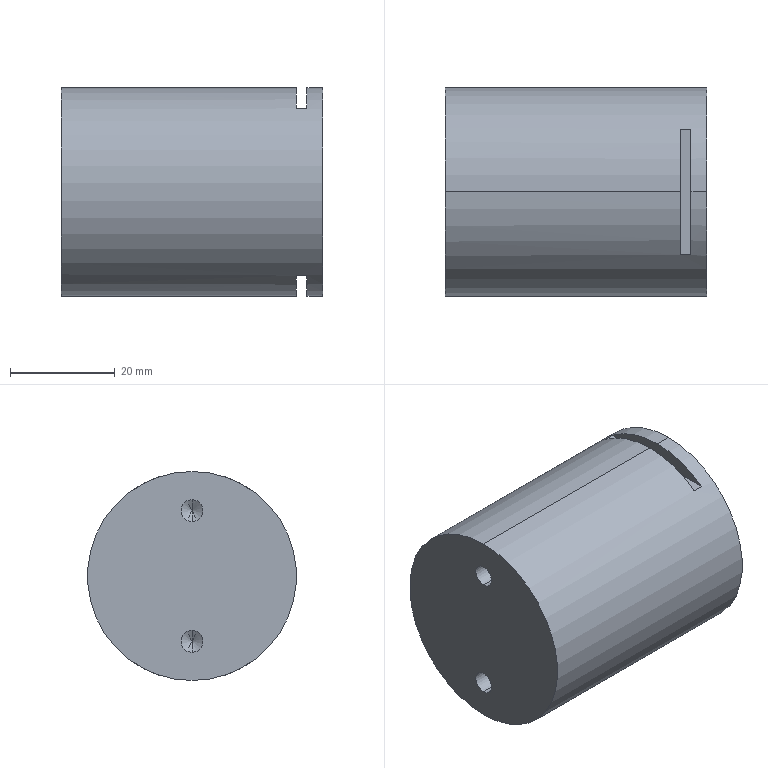Part | STEP file | 01-11 Coil feed support shaft | 1 solid | 18 faces | box 50 x 40 x 40 mm | volume 62215 mm3 | plane 8 | cylinder 6 | cone 4 | commonest cylinder face diameters 4.2 x4 40 x2
STEP:
#1=CARTESIAN_POINT('',(0.,0.,0.));
#2=DIRECTION('',(0.,0.,1.));
#3=DIRECTION('',(1.,0.,0.));
#4=AXIS2_PLACEMENT_3D('',#1,#2,#3);
#5=CARTESIAN_POINT('',(12.4,0.,-10.4));
#6=VERTEX_POINT('',#5);
#7=CARTESIAN_POINT('',(0.,0.,-10.4));
#8=VERTEX_POINT('',#7);
#9=CARTESIAN_POINT('',(12.4,0.,-10.4));
#10=DIRECTION('',(-1.,0.,0.));
#11=VECTOR('',#10,1.);
#12=LINE('',#9,#11);
#13=CARTESIAN_POINT('',(12.4,0.,-12.5));
#14=DIRECTION('',(-1.,0.,0.));
#15=DIRECTION('',(0.,0.,1.));
#16=AXIS2_PLACEMENT_3D('',#13,#14,#15);
#17=CYLINDRICAL_SURFACE('',#16,2.1);
#18=CARTESIAN_POINT('',(6.283,0.));
#19=DIRECTION('',(0.,1.));
#20=VECTOR('',#19,1.);
#21=LINE('',#18,#20);
#22=(GEOMETRIC_REPRESENTATION_CONTEXT(2)PARAMETRIC_REPRESENTATION_CONTEXT()REPRESENTATION_CONTEXT('',''));
#23=DEFINITIONAL_REPRESENTATION('',(#21),#22);
#24=PCURVE('',#17,#23);
#25=CARTESIAN_POINT('',(12.4,0.,-12.5));
#26=DIRECTION('',(-1.,0.,0.));
#27=DIRECTION('',(0.,0.,1.));
#28=AXIS2_PLACEMENT_3D('',#25,#26,#27);
#29=CYLINDRICAL_SURFACE('',#28,2.1);
#30=CARTESIAN_POINT('',(0.,0.));
#31=DIRECTION('',(0.,1.));
#32=VECTOR('',#31,1.);
#33=LINE('',#30,#32);
#34=(GEOMETRIC_REPRESENTATION_CONTEXT(2)PARAMETRIC_REPRESENTATION_CONTEXT()REPRESENTATION_CONTEXT('',''));
#35=DEFINITIONAL_REPRESENTATION('',(#33),#34);
#36=PCURVE('',#29,#35);
#37=SURFACE_CURVE('',#12,(#24,#36),.PCURVE_S1.);
#38=EDGE_CURVE('',#6,#8,#37,.T.);
#39=ORIENTED_EDGE('',*,*,#38,.T.);
#40=CARTESIAN_POINT('',(0.,0.,-14.6));
#41=VERTEX_POINT('',#40);
#42=CARTESIAN_POINT('',(0.,0.,-12.5));
#43=DIRECTION('',(-1.,0.,0.));
#44=DIRECTION('',(0.,0.,1.));
#45=AXIS2_PLACEMENT_3D('',#42,#43,#44);
#46=CIRCLE('',#45,2.1);
#47=CARTESIAN_POINT('',(0.,12.4));
#48=DIRECTION('',(1.,0.));
#49=VECTOR('',#48,1.);
#50=LINE('',#47,#49);
#51=(GEOMETRIC_REPRESENTATION_CONTEXT(2)PARAMETRIC_REPRESENTATION_CONTEXT()REPRESENTATION_CONTEXT('',''));
#52=DEFINITIONAL_REPRESENTATION('',(#50),#51);
#53=PCURVE('',#17,#52);
#54=CARTESIAN_POINT('',(0.,-20.24,20.24));
#55=DIRECTION('',(1.,0.,0.));
#56=DIRECTION('',(0.,0.,-1.));
#57=AXIS2_PLACEMENT_3D('',#54,#55,#56);
#58=PLANE('',#57);
#59=CARTESIAN_POINT('',(30.64,20.24));
#60=CARTESIAN_POINT('',(30.64,23.877));
#61=CARTESIAN_POINT('',(33.79,22.059));
#62=CARTESIAN_POINT('',(36.94,20.24));
#63=CARTESIAN_POINT('',(33.79,18.421));
#64=CARTESIAN_POINT('',(30.64,16.603));
#65=CARTESIAN_POINT('',(30.64,20.24));
#66=(BOUNDED_CURVE()B_SPLINE_CURVE(2,(#59,#60,#61,#62,#63,#64,#65),.UNSPECIFIED.,.T.,.F.)B_SPLINE_CURVE_WITH_KNOTS((1,2,2,2,2,1),(-2.094,0.,2.094,4.189,6.283,8.378),.UNSPECIFIED.)CURVE()GEOMETRIC_REPRESENTATION_ITEM()RATIONAL_B_SPLINE_CURVE((1.,0.5,1.,0.5,1.,0.5,1.))REPRESENTATION_ITEM(''));
#67=(GEOMETRIC_REPRESENTATION_CONTEXT(2)PARAMETRIC_REPRESENTATION_CONTEXT()REPRESENTATION_CONTEXT('',''));
#68=DEFINITIONAL_REPRESENTATION('',(#66),#67);
#69=PCURVE('',#58,#68);
#70=SURFACE_CURVE('',#46,(#53,#69),.PCURVE_S1.);
#71=EDGE_CURVE('',#41,#8,#70,.T.);
#72=ORIENTED_EDGE('',*,*,#71,.F.);
#73=CARTESIAN_POINT('',(12.4,0.,-14.6));
#74=VERTEX_POINT('',#73);
#75=CARTESIAN_POINT('',(12.4,0.,-14.6));
#76=DIRECTION('',(-1.,0.,0.));
#77=VECTOR('',#76,1.);
#78=LINE('',#75,#77);
#79=CARTESIAN_POINT('',(3.142,0.));
#80=DIRECTION('',(0.,1.));
#81=VECTOR('',#80,1.);
#82=LINE('',#79,#81);
#83=(GEOMETRIC_REPRESENTATION_CONTEXT(2)PARAMETRIC_REPRESENTATION_CONTEXT()REPRESENTATION_CONTEXT('',''));
#84=DEFINITIONAL_REPRESENTATION('',(#82),#83);
#85=PCURVE('',#17,#84);
#86=CARTESIAN_POINT('',(3.142,0.));
#87=DIRECTION('',(0.,1.));
#88=VECTOR('',#87,1.);
#89=LINE('',#86,#88);
#90=(GEOMETRIC_REPRESENTATION_CONTEXT(2)PARAMETRIC_REPRESENTATION_CONTEXT()REPRESENTATION_CONTEXT('',''));
#91=DEFINITIONAL_REPRESENTATION('',(#89),#90);
#92=PCURVE('',#29,#91);
#93=SURFACE_CURVE('',#78,(#85,#92),.PCURVE_S1.);
#94=EDGE_CURVE('',#74,#41,#93,.T.);
#95=ORIENTED_EDGE('',*,*,#94,.F.);
#96=CARTESIAN_POINT('',(12.4,0.,-12.5));
#97=DIRECTION('',(1.,0.,0.));
#98=DIRECTION('',(0.,0.,1.));
#99=AXIS2_PLACEMENT_3D('',#96,#97,#98);
#100=CIRCLE('',#99,2.1);
#101=CARTESIAN_POINT('',(6.283,0.));
#102=DIRECTION('',(-1.,0.));
#103=VECTOR('',#102,1.);
#104=LINE('',#101,#103);
#105=(GEOMETRIC_REPRESENTATION_CONTEXT(2)PARAMETRIC_REPRESENTATION_CONTEXT()REPRESENTATION_CONTEXT('',''));
#106=DEFINITIONAL_REPRESENTATION('',(#104),#105);
#107=PCURVE('',#17,#106);
#108=CARTESIAN_POINT('',(-986.338,0.,-12.5));
#109=DIRECTION('',(-1.,0.,0.));
#110=DIRECTION('',(0.,0.,1.));
#111=AXIS2_PLACEMENT_3D('',#108,#109,#110);
#112=CONICAL_SURFACE('',#111,1664.279,1.03);
#113=CARTESIAN_POINT('',(6.283,-998.738));
#114=DIRECTION('',(-1.,0.));
#115=VECTOR('',#114,1.);
#116=LINE('',#113,#115);
#117=(GEOMETRIC_REPRESENTATION_CONTEXT(2)PARAMETRIC_REPRESENTATION_CONTEXT()REPRESENTATION_CONTEXT('',''));
#118=DEFINITIONAL_REPRESENTATION('',(#116),#117);
#119=PCURVE('',#112,#118);
#120=SURFACE_CURVE('',#100,(#107,#119),.PCURVE_S1.);
#121=EDGE_CURVE('',#6,#74,#120,.T.);
#122=ORIENTED_EDGE('',*,*,#121,.F.);
#123=EDGE_LOOP('',(#39,#72,#95,#122));
#124=FACE_BOUND('',#123,.F.);
#125=ADVANCED_FACE('',(#124),#17,.F.);
#126=ORIENTED_EDGE('',*,*,#121,.T.);
#127=CARTESIAN_POINT('',(13.662,0.,-12.5));
#128=VERTEX_POINT('',#127);
#129=CARTESIAN_POINT('',(13.662,0.,-12.5));
#130=DIRECTION('',(-0.515,0.,-0.8572));
#131=VECTOR('',#130,1.);
#132=LINE('',#129,#131);
#133=CARTESIAN_POINT('',(3.142,-1000.));
#134=CARTESIAN_POINT('',(3.142,-999.981));
#135=CARTESIAN_POINT('',(3.142,-999.943));
#136=CARTESIAN_POINT('',(3.142,-999.885));
#137=CARTESIAN_POINT('',(3.142,-999.828));
#138=CARTESIAN_POINT('',(3.142,-999.771));
#139=CARTESIAN_POINT('',(3.142,-999.713));
#140=CARTESIAN_POINT('',(3.142,-999.656));
#141=CARTESIAN_POINT('',(3.142,-999.599));
#142=CARTESIAN_POINT('',(3.142,-999.541));
#143=CARTESIAN_POINT('',(3.142,-999.484));
#144=CARTESIAN_POINT('',(3.142,-999.426));
#145=CARTESIAN_POINT('',(3.142,-999.369));
#146=CARTESIAN_POINT('',(3.142,-999.312));
#147=CARTESIAN_POINT('',(3.142,-999.254));
#148=CARTESIAN_POINT('',(3.142,-999.197));
#149=CARTESIAN_POINT('',(3.142,-999.14));
#150=CARTESIAN_POINT('',(3.142,-999.082));
#151=CARTESIAN_POINT('',(3.142,-999.025));
#152=CARTESIAN_POINT('',(3.142,-998.968));
#153=CARTESIAN_POINT('',(3.142,-998.91));
#154=CARTESIAN_POINT('',(3.142,-998.853));
#155=CARTESIAN_POINT('',(3.142,-998.796));
#156=CARTESIAN_POINT('',(3.142,-998.757));
#157=CARTESIAN_POINT('',(3.142,-998.738));
#158=B_SPLINE_CURVE_WITH_KNOTS('',3,(#133,#134,#135,#136,#137,#138,#139,#140,#141,#142,#143,#144,#145,#146,#147,#148,#149,#150,#151,#152,#153,#154,#155,#156,#157),.UNSPECIFIED.,.F.,.F.,(4,1,1,1,1,1,1,1,1,1,1,1,1,1,1,1,1,1,1,1,1,1,4),(0.,0.1114,0.2227,0.3341,0.4454,0.5568,0.6682,0.7795,0.8909,1.002,1.114,1.225,1.336,1.448,1.559,1.67,1.782,1.893,2.004,2.116,2.227,2.339,2.45),.QUASI_UNIFORM_KNOTS.);
#159=(GEOMETRIC_REPRESENTATION_CONTEXT(2)PARAMETRIC_REPRESENTATION_CONTEXT()REPRESENTATION_CONTEXT('',''));
#160=DEFINITIONAL_REPRESENTATION('',(#158),#159);
#161=PCURVE('',#112,#160);
#162=CARTESIAN_POINT('',(-986.338,0.,-12.5));
#163=DIRECTION('',(-1.,0.,0.));
#164=DIRECTION('',(0.,0.,1.));
#165=AXIS2_PLACEMENT_3D('',#162,#163,#164);
#166=CONICAL_SURFACE('',#165,1664.279,1.03);
#167=CARTESIAN_POINT('',(3.142,-1000.));
#168=CARTESIAN_POINT('',(3.142,-999.981));
#169=CARTESIAN_POINT('',(3.142,-999.943));
#170=CARTESIAN_POINT('',(3.142,-999.885));
#171=CARTESIAN_POINT('',(3.142,-999.828));
#172=CARTESIAN_POINT('',(3.142,-999.771));
#173=CARTESIAN_POINT('',(3.142,-999.713));
#174=CARTESIAN_POINT('',(3.142,-999.656));
#175=CARTESIAN_POINT('',(3.142,-999.599));
#176=CARTESIAN_POINT('',(3.142,-999.541));
#177=CARTESIAN_POINT('',(3.142,-999.484));
#178=CARTESIAN_POINT('',(3.142,-999.426));
#179=CARTESIAN_POINT('',(3.142,-999.369));
#180=CARTESIAN_POINT('',(3.142,-999.312));
#181=CARTESIAN_POINT('',(3.142,-999.254));
#182=CARTESIAN_POINT('',(3.142,-999.197));
#183=CARTESIAN_POINT('',(3.142,-999.14));
#184=CARTESIAN_POINT('',(3.142,-999.082));
#185=CARTESIAN_POINT('',(3.142,-999.025));
#186=CARTESIAN_POINT('',(3.142,-998.968));
#187=CARTESIAN_POINT('',(3.142,-998.91));
#188=CARTESIAN_POINT('',(3.142,-998.853));
#189=CARTESIAN_POINT('',(3.142,-998.796));
#190=CARTESIAN_POINT('',(3.142,-998.757));
#191=CARTESIAN_POINT('',(3.142,-998.738));
#192=B_SPLINE_CURVE_WITH_KNOTS('',3,(#167,#168,#169,#170,#171,#172,#173,#174,#175,#176,#177,#178,#179,#180,#181,#182,#183,#184,#185,#186,#187,#188,#189,#190,#191),.UNSPECIFIED.,.F.,.F.,(4,1,1,1,1,1,1,1,1,1,1,1,1,1,1,1,1,1,1,1,1,1,4),(0.,0.1114,0.2227,0.3341,0.4454,0.5568,0.6682,0.7795,0.8909,1.002,1.114,1.225,1.336,1.448,1.559,1.67,1.782,1.893,2.004,2.116,2.227,2.339,2.45),.QUASI_UNIFORM_KNOTS.);
#193=(GEOMETRIC_REPRESENTATION_CONTEXT(2)PARAMETRIC_REPRESENTATION_CONTEXT()REPRESENTATION_CONTEXT('',''));
#194=DEFINITIONAL_REPRESENTATION('',(#192),#193);
#195=PCURVE('',#166,#194);
#196=SURFACE_CURVE('',#132,(#161,#195),.PCURVE_S1.);
#197=EDGE_CURVE('',#128,#74,#196,.T.);
#198=ORIENTED_EDGE('',*,*,#197,.F.);
#199=CARTESIAN_POINT('',(13.662,0.,-12.5));
#200=DIRECTION('',(-0.515,0.,0.8572));
#201=VECTOR('',#200,1.);
#202=LINE('',#199,#201);
#203=CARTESIAN_POINT('',(6.283,-1000.));
#204=DIRECTION('',(0.,1.));
#205=VECTOR('',#204,1.);
#206=LINE('',#203,#205);
#207=(GEOMETRIC_REPRESENTATION_CONTEXT(2)PARAMETRIC_REPRESENTATION_CONTEXT()REPRESENTATION_CONTEXT('',''));
#208=DEFINITIONAL_REPRESENTATION('',(#206),#207);
#209=PCURVE('',#112,#208);
#210=CARTESIAN_POINT('',(0.,-1000.));
#211=DIRECTION('',(0.,1.));
#212=VECTOR('',#211,1.);
#213=LINE('',#210,#212);
#214=(GEOMETRIC_REPRESENTATION_CONTEXT(2)PARAMETRIC_REPRESENTATION_CONTEXT()REPRESENTATION_CONTEXT('',''));
#215=DEFINITIONAL_REPRESENTATION('',(#213),#214);
#216=PCURVE('',#166,#215);
#217=SURFACE_CURVE('',#202,(#209,#216),.PCURVE_S1.);
#218=EDGE_CURVE('',#128,#6,#217,.T.);
#219=ORIENTED_EDGE('',*,*,#218,.T.);
#220=EDGE_LOOP('',(#126,#198,#219));
#221=FACE_BOUND('',#220,.F.);
#222=ADVANCED_FACE('',(#221),#112,.F.);
#223=CARTESIAN_POINT('',(12.4,0.,14.6));
#224=VERTEX_POINT('',#223);
#225=CARTESIAN_POINT('',(0.,0.,14.6));
#226=VERTEX_POINT('',#225);
#227=CARTESIAN_POINT('',(12.4,0.,14.6));
#228=DIRECTION('',(-1.,0.,0.));
#229=VECTOR('',#228,1.);
#230=LINE('',#227,#229);
#231=CARTESIAN_POINT('',(12.4,0.,12.5));
#232=DIRECTION('',(-1.,0.,0.));
#233=DIRECTION('',(0.,0.,1.));
#234=AXIS2_PLACEMENT_3D('',#231,#232,#233);
#235=CYLINDRICAL_SURFACE('',#234,2.1);
#236=CARTESIAN_POINT('',(6.283,0.));
#237=DIRECTION('',(0.,1.));
#238=VECTOR('',#237,1.);
#239=LINE('',#236,#238);
#240=(GEOMETRIC_REPRESENTATION_CONTEXT(2)PARAMETRIC_REPRESENTATION_CONTEXT()REPRESENTATION_CONTEXT('',''));
#241=DEFINITIONAL_REPRESENTATION('',(#239),#240);
#242=PCURVE('',#235,#241);
#243=CARTESIAN_POINT('',(12.4,0.,12.5));
#244=DIRECTION('',(-1.,0.,0.));
#245=DIRECTION('',(0.,0.,1.));
#246=AXIS2_PLACEMENT_3D('',#243,#244,#245);
#247=CYLINDRICAL_SURFACE('',#246,2.1);
#248=CARTESIAN_POINT('',(0.,0.));
#249=DIRECTION('',(0.,1.));
#250=VECTOR('',#249,1.);
#251=LINE('',#248,#250);
#252=(GEOMETRIC_REPRESENTATION_CONTEXT(2)PARAMETRIC_REPRESENTATION_CONTEXT()REPRESENTATION_CONTEXT('',''));
#253=DEFINITIONAL_REPRESENTATION('',(#251),#252);
#254=PCURVE('',#247,#253);
#255=SURFACE_CURVE('',#230,(#242,#254),.PCURVE_S1.);
#256=EDGE_CURVE('',#224,#226,#255,.T.);
#257=ORIENTED_EDGE('',*,*,#256,.T.);
#258=CARTESIAN_POINT('',(0.,0.,10.4));
#259=VERTEX_POINT('',#258);
#260=CARTESIAN_POINT('',(0.,0.,12.5));
#261=DIRECTION('',(-1.,0.,0.));
#262=DIRECTION('',(0.,0.,1.));
#263=AXIS2_PLACEMENT_3D('',#260,#261,#262);
#264=CIRCLE('',#263,2.1);
#265=CARTESIAN_POINT('',(0.,12.4));
#266=DIRECTION('',(1.,0.));
#267=VECTOR('',#266,1.);
#268=LINE('',#265,#267);
#269=(GEOMETRIC_REPRESENTATION_CONTEXT(2)PARAMETRIC_REPRESENTATION_CONTEXT()REPRESENTATION_CONTEXT('',''));
#270=DEFINITIONAL_REPRESENTATION('',(#268),#269);
#271=PCURVE('',#235,#270);
#272=CARTESIAN_POINT('',(5.64,20.24));
#273=CARTESIAN_POINT('',(5.64,23.877));
#274=CARTESIAN_POINT('',(8.79,22.059));
#275=CARTESIAN_POINT('',(11.94,20.24));
#276=CARTESIAN_POINT('',(8.79,18.421));
#277=CARTESIAN_POINT('',(5.64,16.603));
#278=CARTESIAN_POINT('',(5.64,20.24));
#279=(BOUNDED_CURVE()B_SPLINE_CURVE(2,(#272,#273,#274,#275,#276,#277,#278),.UNSPECIFIED.,.T.,.F.)B_SPLINE_CURVE_WITH_KNOTS((1,2,2,2,2,1),(-2.094,0.,2.094,4.189,6.283,8.378),.UNSPECIFIED.)CURVE()GEOMETRIC_REPRESENTATION_ITEM()RATIONAL_B_SPLINE_CURVE((1.,0.5,1.,0.5,1.,0.5,1.))REPRESENTATION_ITEM(''));
#280=(GEOMETRIC_REPRESENTATION_CONTEXT(2)PARAMETRIC_REPRESENTATION_CONTEXT()REPRESENTATION_CONTEXT('',''));
#281=DEFINITIONAL_REPRESENTATION('',(#279),#280);
#282=PCURVE('',#58,#281);
#283=SURFACE_CURVE('',#264,(#271,#282),.PCURVE_S1.);
#284=EDGE_CURVE('',#259,#226,#283,.T.);
#285=ORIENTED_EDGE('',*,*,#284,.F.);
#286=CARTESIAN_POINT('',(12.4,0.,10.4));
#287=VERTEX_POINT('',#286);
#288=CARTESIAN_POINT('',(12.4,0.,10.4));
#289=DIRECTION('',(-1.,0.,0.));
#290=VECTOR('',#289,1.);
#291=LINE('',#288,#290);
#292=CARTESIAN_POINT('',(3.142,0.));
#293=DIRECTION('',(0.,1.));
#294=VECTOR('',#293,1.);
#295=LINE('',#292,#294);
#296=(GEOMETRIC_REPRESENTATION_CONTEXT(2)PARAMETRIC_REPRESENTATION_CONTEXT()REPRESENTATION_CONTEXT('',''));
#297=DEFINITIONAL_REPRESENTATION('',(#295),#296);
#298=PCURVE('',#235,#297);
#299=CARTESIAN_POINT('',(3.142,0.));
#300=DIRECTION('',(0.,1.));
#301=VECTOR('',#300,1.);
#302=LINE('',#299,#301);
#303=(GEOMETRIC_REPRESENTATION_CONTEXT(2)PARAMETRIC_REPRESENTATION_CONTEXT()REPRESENTATION_CONTEXT('',''));
#304=DEFINITIONAL_REPRESENTATION('',(#302),#303);
#305=PCURVE('',#247,#304);
#306=SURFACE_CURVE('',#291,(#298,#305),.PCURVE_S1.);
#307=EDGE_CURVE('',#287,#259,#306,.T.);
#308=ORIENTED_EDGE('',*,*,#307,.F.);
#309=CARTESIAN_POINT('',(12.4,0.,12.5));
#310=DIRECTION('',(1.,0.,0.));
#311=DIRECTION('',(0.,0.,1.));
#312=AXIS2_PLACEMENT_3D('',#309,#310,#311);
#313=CIRCLE('',#312,2.1);
#314=CARTESIAN_POINT('',(6.283,0.));
#315=DIRECTION('',(-1.,0.));
#316=VECTOR('',#315,1.);
#317=LINE('',#314,#316);
#318=(GEOMETRIC_REPRESENTATION_CONTEXT(2)PARAMETRIC_REPRESENTATION_CONTEXT()REPRESENTATION_CONTEXT('',''));
#319=DEFINITIONAL_REPRESENTATION('',(#317),#318);
#320=PCURVE('',#235,#319);
#321=CARTESIAN_POINT('',(-986.338,0.,12.5));
#322=DIRECTION('',(-1.,0.,0.));
#323=DIRECTION('',(0.,0.,1.));
#324=AXIS2_PLACEMENT_3D('',#321,#322,#323);
#325=CONICAL_SURFACE('',#324,1664.279,1.03);
#326=CARTESIAN_POINT('',(6.283,-998.738));
#327=DIRECTION('',(-1.,0.));
#328=VECTOR('',#327,1.);
#329=LINE('',#326,#328);
#330=(GEOMETRIC_REPRESENTATION_CONTEXT(2)PARAMETRIC_REPRESENTATION_CONTEXT()REPRESENTATION_CONTEXT('',''));
#331=DEFINITIONAL_REPRESENTATION('',(#329),#330);
#332=PCURVE('',#325,#331);
#333=SURFACE_CURVE('',#313,(#320,#332),.PCURVE_S1.);
#334=EDGE_CURVE('',#224,#287,#333,.T.);
#335=ORIENTED_EDGE('',*,*,#334,.F.);
#336=EDGE_LOOP('',(#257,#285,#308,#335));
#337=FACE_BOUND('',#336,.F.);
#338=ADVANCED_FACE('',(#337),#235,.F.);
#339=CARTESIAN_POINT('',(50.,0.,-20.));
#340=VERTEX_POINT('',#339);
#341=CARTESIAN_POINT('',(50.,0.,20.));
#342=VERTEX_POINT('',#341);
#343=CARTESIAN_POINT('',(50.,0.,0.));
#344=DIRECTION('',(1.,0.,0.));
#345=DIRECTION('',(0.,0.,1.));
#346=AXIS2_PLACEMENT_3D('',#343,#344,#345);
#347=CIRCLE('',#346,20.);
#348=CARTESIAN_POINT('',(50.,0.,0.));
#349=DIRECTION('',(-1.,0.,0.));
#350=DIRECTION('',(0.,0.,1.));
#351=AXIS2_PLACEMENT_3D('',#348,#349,#350);
#352=CYLINDRICAL_SURFACE('',#351,20.);
#353=CARTESIAN_POINT('',(6.283,0.));
#354=DIRECTION('',(-1.,0.));
#355=VECTOR('',#354,1.);
#356=LINE('',#353,#355);
#357=(GEOMETRIC_REPRESENTATION_CONTEXT(2)PARAMETRIC_REPRESENTATION_CONTEXT()REPRESENTATION_CONTEXT('',''));
#358=DEFINITIONAL_REPRESENTATION('',(#356),#357);
#359=PCURVE('',#352,#358);
#360=CARTESIAN_POINT('',(50.,-20.24,20.24));
#361=DIRECTION('',(1.,0.,0.));
#362=DIRECTION('',(0.,0.,-1.));
#363=AXIS2_PLACEMENT_3D('',#360,#361,#362);
#364=PLANE('',#363);
#365=CARTESIAN_POINT('',(20.24,20.24));
#366=DIRECTION('',(-1.,0.));
#367=AXIS2_PLACEMENT_2D('',#365,#366);
#368=CIRCLE('',#367,20.);
#369=(GEOMETRIC_REPRESENTATION_CONTEXT(2)PARAMETRIC_REPRESENTATION_CONTEXT()REPRESENTATION_CONTEXT('',''));
#370=DEFINITIONAL_REPRESENTATION('',(#368),#369);
#371=PCURVE('',#364,#370);
#372=SURFACE_CURVE('',#347,(#359,#371),.PCURVE_S1.);
#373=EDGE_CURVE('',#340,#342,#372,.T.);
#374=ORIENTED_EDGE('',*,*,#373,.F.);
#375=CARTESIAN_POINT('',(47.,0.,-20.));
#376=VERTEX_POINT('',#375);
#377=CARTESIAN_POINT('',(50.,0.,-20.));
#378=DIRECTION('',(-1.,0.,0.));
#379=VECTOR('',#378,1.);
#380=LINE('',#377,#379);
#381=CARTESIAN_POINT('',(3.142,0.));
#382=DIRECTION('',(0.,1.));
#383=VECTOR('',#382,1.);
#384=LINE('',#381,#383);
#385=(GEOMETRIC_REPRESENTATION_CONTEXT(2)PARAMETRIC_REPRESENTATION_CONTEXT()REPRESENTATION_CONTEXT('',''));
#386=DEFINITIONAL_REPRESENTATION('',(#384),#385);
#387=PCURVE('',#352,#386);
#388=CARTESIAN_POINT('',(50.,0.,0.));
#389=DIRECTION('',(-1.,0.,0.));
#390=DIRECTION('',(0.,0.,1.));
#391=AXIS2_PLACEMENT_3D('',#388,#389,#390);
#392=CYLINDRICAL_SURFACE('',#391,20.);
#393=CARTESIAN_POINT('',(3.142,0.));
#394=DIRECTION('',(0.,1.));
#395=VECTOR('',#394,1.);
#396=LINE('',#393,#395);
#397=(GEOMETRIC_REPRESENTATION_CONTEXT(2)PARAMETRIC_REPRESENTATION_CONTEXT()REPRESENTATION_CONTEXT('',''));
#398=DEFINITIONAL_REPRESENTATION('',(#396),#397);
#399=PCURVE('',#392,#398);
#400=SURFACE_CURVE('',#380,(#387,#399),.PCURVE_S1.);
#401=EDGE_CURVE('',#340,#376,#400,.T.);
#402=ORIENTED_EDGE('',*,*,#401,.T.);
#403=CARTESIAN_POINT('',(47.,12.,-16.));
#404=VERTEX_POINT('',#403);
#405=CARTESIAN_POINT('',(47.,0.,0.));
#406=DIRECTION('',(-1.,0.,0.));
#407=DIRECTION('',(0.,0.,1.));
#408=AXIS2_PLACEMENT_3D('',#405,#406,#407);
#409=CIRCLE('',#408,20.);
#410=CARTESIAN_POINT('',(0.,3.));
#411=DIRECTION('',(1.,0.));
#412=VECTOR('',#411,1.);
#413=LINE('',#410,#412);
#414=(GEOMETRIC_REPRESENTATION_CONTEXT(2)PARAMETRIC_REPRESENTATION_CONTEXT()REPRESENTATION_CONTEXT('',''));
#415=DEFINITIONAL_REPRESENTATION('',(#413),#414);
#416=PCURVE('',#352,#415);
#417=CARTESIAN_POINT('',(47.,-12.144,-16.));
#418=DIRECTION('',(1.,0.,0.));
#419=DIRECTION('',(0.,0.,-1.));
#420=AXIS2_PLACEMENT_3D('',#417,#418,#419);
#421=PLANE('',#420);
#422=CARTESIAN_POINT('',(-36.,12.144));
#423=CARTESIAN_POINT('',(-36.,46.785));
#424=CARTESIAN_POINT('',(-6.,29.465));
#425=CARTESIAN_POINT('',(24.,12.144));
#426=CARTESIAN_POINT('',(-6.,-5.177));
#427=CARTESIAN_POINT('',(-36.,-22.497));
#428=CARTESIAN_POINT('',(-36.,12.144));
#429=(BOUNDED_CURVE()B_SPLINE_CURVE(2,(#422,#423,#424,#425,#426,#427,#428),.UNSPECIFIED.,.T.,.F.)B_SPLINE_CURVE_WITH_KNOTS((1,2,2,2,2,1),(-2.094,0.,2.094,4.189,6.283,8.378),.UNSPECIFIED.)CURVE()GEOMETRIC_REPRESENTATION_ITEM()RATIONAL_B_SPLINE_CURVE((1.,0.5,1.,0.5,1.,0.5,1.))REPRESENTATION_ITEM(''));
#430=(GEOMETRIC_REPRESENTATION_CONTEXT(2)PARAMETRIC_REPRESENTATION_CONTEXT()REPRESENTATION_CONTEXT('',''));
#431=DEFINITIONAL_REPRESENTATION('',(#429),#430);
#432=PCURVE('',#421,#431);
#433=SURFACE_CURVE('',#409,(#416,#432),.PCURVE_S1.);
#434=EDGE_CURVE('',#404,#376,#433,.T.);
#435=ORIENTED_EDGE('',*,*,#434,.F.);
#436=CARTESIAN_POINT('',(45.,12.,-16.));
#437=VERTEX_POINT('',#436);
#438=CARTESIAN_POINT('',(25.,12.,-16.));
#439=DIRECTION('',(1.,0.,0.));
#440=VECTOR('',#439,1.);
#441=LINE('',#438,#440);
#442=CARTESIAN_POINT('',(2.498,25.));
#443=DIRECTION('',(0.,-1.));
#444=VECTOR('',#443,1.);
#445=LINE('',#442,#444);
#446=(GEOMETRIC_REPRESENTATION_CONTEXT(2)PARAMETRIC_REPRESENTATION_CONTEXT()REPRESENTATION_CONTEXT('',''));
#447=DEFINITIONAL_REPRESENTATION('',(#445),#446);
#448=PCURVE('',#352,#447);
#449=CARTESIAN_POINT('',(45.,-12.,-16.));
#450=DIRECTION('',(0.,0.,1.));
#451=DIRECTION('',(1.,0.,0.));
#452=AXIS2_PLACEMENT_3D('',#449,#450,#451);
#453=PLANE('',#452);
#454=CARTESIAN_POINT('',(-20.,24.));
#455=DIRECTION('',(1.,0.));
#456=VECTOR('',#455,1.);
#457=LINE('',#454,#456);
#458=(GEOMETRIC_REPRESENTATION_CONTEXT(2)PARAMETRIC_REPRESENTATION_CONTEXT()REPRESENTATION_CONTEXT('',''));
#459=DEFINITIONAL_REPRESENTATION('',(#457),#458);
#460=PCURVE('',#453,#459);
#461=SURFACE_CURVE('',#441,(#448,#460),.PCURVE_S1.);
#462=EDGE_CURVE('',#437,#404,#461,.T.);
#463=ORIENTED_EDGE('',*,*,#462,.F.);
#464=CARTESIAN_POINT('',(45.,0.,-20.));
#465=VERTEX_POINT('',#464);
#466=CARTESIAN_POINT('',(45.,0.,0.));
#467=DIRECTION('',(1.,0.,0.));
#468=DIRECTION('',(0.,0.,1.));
#469=AXIS2_PLACEMENT_3D('',#466,#467,#468);
#470=CIRCLE('',#469,20.);
#471=CARTESIAN_POINT('',(6.283,5.));
#472=DIRECTION('',(-1.,0.));
#473=VECTOR('',#472,1.);
#474=LINE('',#471,#473);
#475=(GEOMETRIC_REPRESENTATION_CONTEXT(2)PARAMETRIC_REPRESENTATION_CONTEXT()REPRESENTATION_CONTEXT('',''));
#476=DEFINITIONAL_REPRESENTATION('',(#474),#475);
#477=PCURVE('',#352,#476);
#478=CARTESIAN_POINT('',(45.,-12.144,-20.024));
#479=DIRECTION('',(-1.,0.,0.));
#480=DIRECTION('',(0.,0.,1.));
#481=AXIS2_PLACEMENT_3D('',#478,#479,#480);
#482=PLANE('',#481);
#483=CARTESIAN_POINT('',(40.024,12.144));
#484=CARTESIAN_POINT('',(40.024,-22.497));
#485=CARTESIAN_POINT('',(10.024,-5.177));
#486=CARTESIAN_POINT('',(-19.976,12.144));
#487=CARTESIAN_POINT('',(10.024,29.465));
#488=CARTESIAN_POINT('',(40.024,46.785));
#489=CARTESIAN_POINT('',(40.024,12.144));
#490=(BOUNDED_CURVE()B_SPLINE_CURVE(2,(#483,#484,#485,#486,#487,#488,#489),.UNSPECIFIED.,.T.,.F.)B_SPLINE_CURVE_WITH_KNOTS((1,2,2,2,2,1),(-2.094,0.,2.094,4.189,6.283,8.378),.UNSPECIFIED.)CURVE()GEOMETRIC_REPRESENTATION_ITEM()RATIONAL_B_SPLINE_CURVE((1.,0.5,1.,0.5,1.,0.5,1.))REPRESENTATION_ITEM(''));
#491=(GEOMETRIC_REPRESENTATION_CONTEXT(2)PARAMETRIC_REPRESENTATION_CONTEXT()REPRESENTATION_CONTEXT('',''));
#492=DEFINITIONAL_REPRESENTATION('',(#490),#491);
#493=PCURVE('',#482,#492);
#494=SURFACE_CURVE('',#470,(#477,#493),.PCURVE_S1.);
#495=EDGE_CURVE('',#465,#437,#494,.T.);
#496=ORIENTED_EDGE('',*,*,#495,.F.);
#497=CARTESIAN_POINT('',(0.,0.,-20.));
#498=VERTEX_POINT('',#497);
#499=CARTESIAN_POINT('',(50.,0.,-20.));
#500=DIRECTION('',(-1.,0.,0.));
#501=VECTOR('',#500,1.);
#502=LINE('',#499,#501);
#503=CARTESIAN_POINT('',(3.142,0.));
#504=DIRECTION('',(0.,1.));
#505=VECTOR('',#504,1.);
#506=LINE('',#503,#505);
#507=(GEOMETRIC_REPRESENTATION_CONTEXT(2)PARAMETRIC_REPRESENTATION_CONTEXT()REPRESENTATION_CONTEXT('',''));
#508=DEFINITIONAL_REPRESENTATION('',(#506),#507);
#509=PCURVE('',#352,#508);
#510=CARTESIAN_POINT('',(3.142,0.));
#511=DIRECTION('',(0.,1.));
#512=VECTOR('',#511,1.);
#513=LINE('',#510,#512);
#514=(GEOMETRIC_REPRESENTATION_CONTEXT(2)PARAMETRIC_REPRESENTATION_CONTEXT()REPRESENTATION_CONTEXT('',''));
#515=DEFINITIONAL_REPRESENTATION('',(#513),#514);
#516=PCURVE('',#392,#515);
#517=SURFACE_CURVE('',#502,(#509,#516),.PCURVE_S1.);
#518=EDGE_CURVE('',#465,#498,#517,.T.);
#519=ORIENTED_EDGE('',*,*,#518,.T.);
#520=CARTESIAN_POINT('',(0.,0.,20.));
#521=VERTEX_POINT('',#520);
#522=CARTESIAN_POINT('',(0.,0.,0.));
#523=DIRECTION('',(1.,0.,0.));
#524=DIRECTION('',(0.,0.,1.));
#525=AXIS2_PLACEMENT_3D('',#522,#523,#524);
#526=CIRCLE('',#525,20.);
#527=CARTESIAN_POINT('',(6.283,50.));
#528=DIRECTION('',(-1.,0.));
#529=VECTOR('',#528,1.);
#530=LINE('',#527,#529);
#531=(GEOMETRIC_REPRESENTATION_CONTEXT(2)PARAMETRIC_REPRESENTATION_CONTEXT()REPRESENTATION_CONTEXT('',''));
#532=DEFINITIONAL_REPRESENTATION('',(#530),#531);
#533=PCURVE('',#352,#532);
#534=CARTESIAN_POINT('',(20.24,20.24));
#535=DIRECTION('',(-1.,0.));
#536=AXIS2_PLACEMENT_2D('',#534,#535);
#537=CIRCLE('',#536,20.);
#538=(GEOMETRIC_REPRESENTATION_CONTEXT(2)PARAMETRIC_REPRESENTATION_CONTEXT()REPRESENTATION_CONTEXT('',''));
#539=DEFINITIONAL_REPRESENTATION('',(#537),#538);
#540=PCURVE('',#58,#539);
#541=SURFACE_CURVE('',#526,(#533,#540),.PCURVE_S1.);
#542=EDGE_CURVE('',#498,#521,#541,.T.);
#543=ORIENTED_EDGE('',*,*,#542,.T.);
#544=CARTESIAN_POINT('',(45.,0.,20.));
#545=VERTEX_POINT('',#544);
#546=CARTESIAN_POINT('',(50.,0.,20.));
#547=DIRECTION('',(-1.,0.,0.));
#548=VECTOR('',#547,1.);
#549=LINE('',#546,#548);
#550=CARTESIAN_POINT('',(0.,0.));
#551=DIRECTION('',(0.,1.));
#552=VECTOR('',#551,1.);
#553=LINE('',#550,#552);
#554=(GEOMETRIC_REPRESENTATION_CONTEXT(2)PARAMETRIC_REPRESENTATION_CONTEXT()REPRESENTATION_CONTEXT('',''));
#555=DEFINITIONAL_REPRESENTATION('',(#553),#554);
#556=PCURVE('',#352,#555);
#557=CARTESIAN_POINT('',(6.283,0.));
#558=DIRECTION('',(0.,1.));
#559=VECTOR('',#558,1.);
#560=LINE('',#557,#559);
#561=(GEOMETRIC_REPRESENTATION_CONTEXT(2)PARAMETRIC_REPRESENTATION_CONTEXT()REPRESENTATION_CONTEXT('',''));
#562=DEFINITIONAL_REPRESENTATION('',(#560),#561);
#563=PCURVE('',#392,#562);
#564=SURFACE_CURVE('',#549,(#556,#563),.PCURVE_S1.);
#565=EDGE_CURVE('',#545,#521,#564,.T.);
#566=ORIENTED_EDGE('',*,*,#565,.F.);
#567=CARTESIAN_POINT('',(45.,12.,16.));
#568=VERTEX_POINT('',#567);
#569=CARTESIAN_POINT('',(45.,0.,0.));
#570=DIRECTION('',(1.,0.,0.));
#571=DIRECTION('',(0.,0.,1.));
#572=AXIS2_PLACEMENT_3D('',#569,#570,#571);
#573=CIRCLE('',#572,20.);
#574=CARTESIAN_POINT('',(6.283,5.));
#575=DIRECTION('',(-1.,0.));
#576=VECTOR('',#575,1.);
#577=LINE('',#574,#576);
#578=(GEOMETRIC_REPRESENTATION_CONTEXT(2)PARAMETRIC_REPRESENTATION_CONTEXT()REPRESENTATION_CONTEXT('',''));
#579=DEFINITIONAL_REPRESENTATION('',(#577),#578);
#580=PCURVE('',#352,#579);
#581=CARTESIAN_POINT('',(45.,-12.144,16.));
#582=DIRECTION('',(-1.,0.,0.));
#583=DIRECTION('',(0.,0.,1.));
#584=AXIS2_PLACEMENT_3D('',#581,#582,#583);
#585=PLANE('',#584);
#586=CARTESIAN_POINT('',(4.,12.144));
#587=CARTESIAN_POINT('',(4.,-22.497));
#588=CARTESIAN_POINT('',(-26.,-5.177));
#589=CARTESIAN_POINT('',(-56.,12.144));
#590=CARTESIAN_POINT('',(-26.,29.465));
#591=CARTESIAN_POINT('',(4.,46.785));
#592=CARTESIAN_POINT('',(4.,12.144));
#593=(BOUNDED_CURVE()B_SPLINE_CURVE(2,(#586,#587,#588,#589,#590,#591,#592),.UNSPECIFIED.,.T.,.F.)B_SPLINE_CURVE_WITH_KNOTS((1,2,2,2,2,1),(-2.094,0.,2.094,4.189,6.283,8.378),.UNSPECIFIED.)CURVE()GEOMETRIC_REPRESENTATION_ITEM()RATIONAL_B_SPLINE_CURVE((1.,0.5,1.,0.5,1.,0.5,1.))REPRESENTATION_ITEM(''));
#594=(GEOMETRIC_REPRESENTATION_CONTEXT(2)PARAMETRIC_REPRESENTATION_CONTEXT()REPRESENTATION_CONTEXT('',''));
#595=DEFINITIONAL_REPRESENTATION('',(#593),#594);
#596=PCURVE('',#585,#595);
#597=SURFACE_CURVE('',#573,(#580,#596),.PCURVE_S1.);
#598=EDGE_CURVE('',#568,#545,#597,.T.);
#599=ORIENTED_EDGE('',*,*,#598,.F.);
#600=CARTESIAN_POINT('',(47.,12.,16.));
#601=VERTEX_POINT('',#600);
#602=CARTESIAN_POINT('',(25.,12.,16.));
#603=DIRECTION('',(-1.,0.,0.));
#604=VECTOR('',#603,1.);
#605=LINE('',#602,#604);
#606=CARTESIAN_POINT('',(0.6435,25.));
#607=DIRECTION('',(0.,1.));
#608=VECTOR('',#607,1.);
#609=LINE('',#606,#608);
#610=(GEOMETRIC_REPRESENTATION_CONTEXT(2)PARAMETRIC_REPRESENTATION_CONTEXT()REPRESENTATION_CONTEXT('',''));
#611=DEFINITIONAL_REPRESENTATION('',(#609),#610);
#612=PCURVE('',#352,#611);
#613=CARTESIAN_POINT('',(47.,-12.,16.));
#614=DIRECTION('',(0.,0.,-1.));
#615=DIRECTION('',(-1.,0.,0.));
#616=AXIS2_PLACEMENT_3D('',#613,#614,#615);
#617=PLANE('',#616);
#618=CARTESIAN_POINT('',(22.,24.));
#619=DIRECTION('',(1.,0.));
#620=VECTOR('',#619,1.);
#621=LINE('',#618,#620);
#622=(GEOMETRIC_REPRESENTATION_CONTEXT(2)PARAMETRIC_REPRESENTATION_CONTEXT()REPRESENTATION_CONTEXT('',''));
#623=DEFINITIONAL_REPRESENTATION('',(#621),#622);
#624=PCURVE('',#617,#623);
#625=SURFACE_CURVE('',#605,(#612,#624),.PCURVE_S1.);
#626=EDGE_CURVE('',#601,#568,#625,.T.);
#627=ORIENTED_EDGE('',*,*,#626,.F.);
#628=CARTESIAN_POINT('',(47.,0.,20.));
#629=VERTEX_POINT('',#628);
#630=CARTESIAN_POINT('',(47.,0.,0.));
#631=DIRECTION('',(-1.,0.,0.));
#632=DIRECTION('',(0.,0.,1.));
#633=AXIS2_PLACEMENT_3D('',#630,#631,#632);
#634=CIRCLE('',#633,20.);
#635=CARTESIAN_POINT('',(0.,3.));
#636=DIRECTION('',(1.,0.));
#637=VECTOR('',#636,1.);
#638=LINE('',#635,#637);
#639=(GEOMETRIC_REPRESENTATION_CONTEXT(2)PARAMETRIC_REPRESENTATION_CONTEXT()REPRESENTATION_CONTEXT('',''));
#640=DEFINITIONAL_REPRESENTATION('',(#638),#639);
#641=PCURVE('',#352,#640);
#642=CARTESIAN_POINT('',(47.,-12.144,20.024));
#643=DIRECTION('',(1.,0.,0.));
#644=DIRECTION('',(0.,0.,-1.));
#645=AXIS2_PLACEMENT_3D('',#642,#643,#644);
#646=PLANE('',#645);
#647=CARTESIAN_POINT('',(0.024,12.144));
#648=CARTESIAN_POINT('',(0.024,46.785));
#649=CARTESIAN_POINT('',(30.024,29.465));
#650=CARTESIAN_POINT('',(60.024,12.144));
#651=CARTESIAN_POINT('',(30.024,-5.177));
#652=CARTESIAN_POINT('',(0.024,-22.497));
#653=CARTESIAN_POINT('',(0.024,12.144));
#654=(BOUNDED_CURVE()B_SPLINE_CURVE(2,(#647,#648,#649,#650,#651,#652,#653),.UNSPECIFIED.,.T.,.F.)B_SPLINE_CURVE_WITH_KNOTS((1,2,2,2,2,1),(-2.094,0.,2.094,4.189,6.283,8.378),.UNSPECIFIED.)CURVE()GEOMETRIC_REPRESENTATION_ITEM()RATIONAL_B_SPLINE_CURVE((1.,0.5,1.,0.5,1.,0.5,1.))REPRESENTATION_ITEM(''));
#655=(GEOMETRIC_REPRESENTATION_CONTEXT(2)PARAMETRIC_REPRESENTATION_CONTEXT()REPRESENTATION_CONTEXT('',''));
#656=DEFINITIONAL_REPRESENTATION('',(#654),#655);
#657=PCURVE('',#646,#656);
#658=SURFACE_CURVE('',#634,(#641,#657),.PCURVE_S1.);
#659=EDGE_CURVE('',#629,#601,#658,.T.);
#660=ORIENTED_EDGE('',*,*,#659,.F.);
#661=CARTESIAN_POINT('',(50.,0.,20.));
#662=DIRECTION('',(-1.,0.,0.));
#663=VECTOR('',#662,1.);
#664=LINE('',#661,#663);
#665=CARTESIAN_POINT('',(0.,0.));
#666=DIRECTION('',(0.,1.));
#667=VECTOR('',#666,1.);
#668=LINE('',#665,#667);
#669=(GEOMETRIC_REPRESENTATION_CONTEXT(2)PARAMETRIC_REPRESENTATION_CONTEXT()REPRESENTATION_CONTEXT('',''));
#670=DEFINITIONAL_REPRESENTATION('',(#668),#669);
#671=PCURVE('',#352,#670);
#672=CARTESIAN_POINT('',(6.283,0.));
#673=DIRECTION('',(0.,1.));
#674=VECTOR('',#673,1.);
#675=LINE('',#672,#674);
#676=(GEOMETRIC_REPRESENTATION_CONTEXT(2)PARAMETRIC_REPRESENTATION_CONTEXT()REPRESENTATION_CONTEXT('',''));
#677=DEFINITIONAL_REPRESENTATION('',(#675),#676);
#678=PCURVE('',#392,#677);
#679=SURFACE_CURVE('',#664,(#671,#678),.PCURVE_S1.);
#680=EDGE_CURVE('',#342,#629,#679,.T.);
#681=ORIENTED_EDGE('',*,*,#680,.F.);
#682=EDGE_LOOP('',(#374,#402,#435,#463,#496,#519,#543,#566,#599,#627,#660,#681));
#683=FACE_BOUND('',#682,.T.);
#684=ADVANCED_FACE('',(#683),#352,.T.);
#685=ORIENTED_EDGE('',*,*,#334,.T.);
#686=CARTESIAN_POINT('',(13.662,0.,12.5));
#687=VERTEX_POINT('',#686);
#688=CARTESIAN_POINT('',(13.662,0.,12.5));
#689=DIRECTION('',(-0.515,0.,-0.8572));
#690=VECTOR('',#689,1.);
#691=LINE('',#688,#690);
#692=CARTESIAN_POINT('',(3.142,-1000.));
#693=CARTESIAN_POINT('',(3.142,-999.981));
#694=CARTESIAN_POINT('',(3.142,-999.943));
#695=CARTESIAN_POINT('',(3.142,-999.885));
#696=CARTESIAN_POINT('',(3.142,-999.828));
#697=CARTESIAN_POINT('',(3.142,-999.771));
#698=CARTESIAN_POINT('',(3.142,-999.713));
#699=CARTESIAN_POINT('',(3.142,-999.656));
#700=CARTESIAN_POINT('',(3.142,-999.599));
#701=CARTESIAN_POINT('',(3.142,-999.541));
#702=CARTESIAN_POINT('',(3.142,-999.484));
#703=CARTESIAN_POINT('',(3.142,-999.426));
#704=CARTESIAN_POINT('',(3.142,-999.369));
#705=CARTESIAN_POINT('',(3.142,-999.312));
#706=CARTESIAN_POINT('',(3.142,-999.254));
#707=CARTESIAN_POINT('',(3.142,-999.197));
#708=CARTESIAN_POINT('',(3.142,-999.14));
#709=CARTESIAN_POINT('',(3.142,-999.082));
#710=CARTESIAN_POINT('',(3.142,-999.025));
#711=CARTESIAN_POINT('',(3.142,-998.968));
#712=CARTESIAN_POINT('',(3.142,-998.91));
#713=CARTESIAN_POINT('',(3.142,-998.853));
#714=CARTESIAN_POINT('',(3.142,-998.796));
#715=CARTESIAN_POINT('',(3.142,-998.757));
#716=CARTESIAN_POINT('',(3.142,-998.738));
#717=B_SPLINE_CURVE_WITH_KNOTS('',3,(#692,#693,#694,#695,#696,#697,#698,#699,#700,#701,#702,#703,#704,#705,#706,#707,#708,#709,#710,#711,#712,#713,#714,#715,#716),.UNSPECIFIED.,.F.,.F.,(4,1,1,1,1,1,1,1,1,1,1,1,1,1,1,1,1,1,1,1,1,1,4),(0.,0.1114,0.2227,0.3341,0.4454,0.5568,0.6682,0.7795,0.8909,1.002,1.114,1.225,1.336,1.448,1.559,1.67,1.782,1.893,2.004,2.116,2.227,2.339,2.45),.QUASI_UNIFORM_KNOTS.);
#718=(GEOMETRIC_REPRESENTATION_CONTEXT(2)PARAMETRIC_REPRESENTATION_CONTEXT()REPRESENTATION_CONTEXT('',''));
#719=DEFINITIONAL_REPRESENTATION('',(#717),#718);
#720=PCURVE('',#325,#719);
#721=CARTESIAN_POINT('',(-986.338,0.,12.5));
#722=DIRECTION('',(-1.,0.,0.));
#723=DIRECTION('',(0.,0.,1.));
#724=AXIS2_PLACEMENT_3D('',#721,#722,#723);
#725=CONICAL_SURFACE('',#724,1664.279,1.03);
#726=CARTESIAN_POINT('',(3.142,-1000.));
#727=CARTESIAN_POINT('',(3.142,-999.981));
#728=CARTESIAN_POINT('',(3.142,-999.943));
#729=CARTESIAN_POINT('',(3.142,-999.885));
#730=CARTESIAN_POINT('',(3.142,-999.828));
#731=CARTESIAN_POINT('',(3.142,-999.771));
#732=CARTESIAN_POINT('',(3.142,-999.713));
#733=CARTESIAN_POINT('',(3.142,-999.656));
#734=CARTESIAN_POINT('',(3.142,-999.599));
#735=CARTESIAN_POINT('',(3.142,-999.541));
#736=CARTESIAN_POINT('',(3.142,-999.484));
#737=CARTESIAN_POINT('',(3.142,-999.426));
#738=CARTESIAN_POINT('',(3.142,-999.369));
#739=CARTESIAN_POINT('',(3.142,-999.312));
#740=CARTESIAN_POINT('',(3.142,-999.254));
#741=CARTESIAN_POINT('',(3.142,-999.197));
#742=CARTESIAN_POINT('',(3.142,-999.14));
#743=CARTESIAN_POINT('',(3.142,-999.082));
#744=CARTESIAN_POINT('',(3.142,-999.025));
#745=CARTESIAN_POINT('',(3.142,-998.968));
#746=CARTESIAN_POINT('',(3.142,-998.91));
#747=CARTESIAN_POINT('',(3.142,-998.853));
#748=CARTESIAN_POINT('',(3.142,-998.796));
#749=CARTESIAN_POINT('',(3.142,-998.757));
#750=CARTESIAN_POINT('',(3.142,-998.738));
#751=B_SPLINE_CURVE_WITH_KNOTS('',3,(#726,#727,#728,#729,#730,#731,#732,#733,#734,#735,#736,#737,#738,#739,#740,#741,#742,#743,#744,#745,#746,#747,#748,#749,#750),.UNSPECIFIED.,.F.,.F.,(4,1,1,1,1,1,1,1,1,1,1,1,1,1,1,1,1,1,1,1,1,1,4),(0.,0.1114,0.2227,0.3341,0.4454,0.5568,0.6682,0.7795,0.8909,1.002,1.114,1.225,1.336,1.448,1.559,1.67,1.782,1.893,2.004,2.116,2.227,2.339,2.45),.QUASI_UNIFORM_KNOTS.);
#752=(GEOMETRIC_REPRESENTATION_CONTEXT(2)PARAMETRIC_REPRESENTATION_CONTEXT()REPRESENTATION_CONTEXT('',''));
#753=DEFINITIONAL_REPRESENTATION('',(#751),#752);
#754=PCURVE('',#725,#753);
#755=SURFACE_CURVE('',#691,(#720,#754),.PCURVE_S1.);
#756=EDGE_CURVE('',#687,#287,#755,.T.);
#757=ORIENTED_EDGE('',*,*,#756,.F.);
#758=CARTESIAN_POINT('',(13.662,0.,12.5));
#759=DIRECTION('',(-0.515,0.,0.8572));
#760=VECTOR('',#759,1.);
#761=LINE('',#758,#760);
#762=CARTESIAN_POINT('',(6.283,-1000.));
#763=DIRECTION('',(0.,1.));
#764=VECTOR('',#763,1.);
#765=LINE('',#762,#764);
#766=(GEOMETRIC_REPRESENTATION_CONTEXT(2)PARAMETRIC_REPRESENTATION_CONTEXT()REPRESENTATION_CONTEXT('',''));
#767=DEFINITIONAL_REPRESENTATION('',(#765),#766);
#768=PCURVE('',#325,#767);
#769=CARTESIAN_POINT('',(0.,-1000.));
#770=DIRECTION('',(0.,1.));
#771=VECTOR('',#770,1.);
#772=LINE('',#769,#771);
#773=(GEOMETRIC_REPRESENTATION_CONTEXT(2)PARAMETRIC_REPRESENTATION_CONTEXT()REPRESENTATION_CONTEXT('',''));
#774=DEFINITIONAL_REPRESENTATION('',(#772),#773);
#775=PCURVE('',#725,#774);
#776=SURFACE_CURVE('',#761,(#768,#775),.PCURVE_S1.);
#777=EDGE_CURVE('',#687,#224,#776,.T.);
#778=ORIENTED_EDGE('',*,*,#777,.T.);
#779=EDGE_LOOP('',(#685,#757,#778));
#780=FACE_BOUND('',#779,.F.);
#781=ADVANCED_FACE('',(#780),#325,.F.);
#782=CARTESIAN_POINT('',(0.,0.,-12.5));
#783=DIRECTION('',(-1.,0.,0.));
#784=DIRECTION('',(0.,0.,1.));
#785=AXIS2_PLACEMENT_3D('',#782,#783,#784);
#786=CIRCLE('',#785,2.1);
#787=CARTESIAN_POINT('',(0.,12.4));
#788=DIRECTION('',(1.,0.));
#789=VECTOR('',#788,1.);
#790=LINE('',#787,#789);
#791=(GEOMETRIC_REPRESENTATION_CONTEXT(2)PARAMETRIC_REPRESENTATION_CONTEXT()REPRESENTATION_CONTEXT('',''));
#792=DEFINITIONAL_REPRESENTATION('',(#790),#791);
#793=PCURVE('',#29,#792);
#794=CARTESIAN_POINT('',(30.64,20.24));
#795=CARTESIAN_POINT('',(30.64,23.877));
#796=CARTESIAN_POINT('',(33.79,22.059));
#797=CARTESIAN_POINT('',(36.94,20.24));
#798=CARTESIAN_POINT('',(33.79,18.421));
#799=CARTESIAN_POINT('',(30.64,16.603));
#800=CARTESIAN_POINT('',(30.64,20.24));
#801=(BOUNDED_CURVE()B_SPLINE_CURVE(2,(#794,#795,#796,#797,#798,#799,#800),.UNSPECIFIED.,.T.,.F.)B_SPLINE_CURVE_WITH_KNOTS((1,2,2,2,2,1),(-2.094,0.,2.094,4.189,6.283,8.378),.UNSPECIFIED.)CURVE()GEOMETRIC_REPRESENTATION_ITEM()RATIONAL_B_SPLINE_CURVE((1.,0.5,1.,0.5,1.,0.5,1.))REPRESENTATION_ITEM(''));
#802=(GEOMETRIC_REPRESENTATION_CONTEXT(2)PARAMETRIC_REPRESENTATION_CONTEXT()REPRESENTATION_CONTEXT('',''));
#803=DEFINITIONAL_REPRESENTATION('',(#801),#802);
#804=PCURVE('',#58,#803);
#805=SURFACE_CURVE('',#786,(#793,#804),.PCURVE_S1.);
#806=EDGE_CURVE('',#8,#41,#805,.T.);
#807=ORIENTED_EDGE('',*,*,#806,.F.);
#808=ORIENTED_EDGE('',*,*,#38,.F.);
#809=CARTESIAN_POINT('',(12.4,0.,-12.5));
#810=DIRECTION('',(1.,0.,0.));
#811=DIRECTION('',(0.,0.,1.));
#812=AXIS2_PLACEMENT_3D('',#809,#810,#811);
#813=CIRCLE('',#812,2.1);
#814=CARTESIAN_POINT('',(6.283,0.));
#815=DIRECTION('',(-1.,0.));
#816=VECTOR('',#815,1.);
#817=LINE('',#814,#816);
#818=(GEOMETRIC_REPRESENTATION_CONTEXT(2)PARAMETRIC_REPRESENTATION_CONTEXT()REPRESENTATION_CONTEXT('',''));
#819=DEFINITIONAL_REPRESENTATION('',(#817),#818);
#820=PCURVE('',#29,#819);
#821=CARTESIAN_POINT('',(6.283,-998.738));
#822=DIRECTION('',(-1.,0.));
#823=VECTOR('',#822,1.);
#824=LINE('',#821,#823);
#825=(GEOMETRIC_REPRESENTATION_CONTEXT(2)PARAMETRIC_REPRESENTATION_CONTEXT()REPRESENTATION_CONTEXT('',''));
#826=DEFINITIONAL_REPRESENTATION('',(#824),#825);
#827=PCURVE('',#166,#826);
#828=SURFACE_CURVE('',#813,(#820,#827),.PCURVE_S1.);
#829=EDGE_CURVE('',#74,#6,#828,.T.);
#830=ORIENTED_EDGE('',*,*,#829,.F.);
#831=ORIENTED_EDGE('',*,*,#94,.T.);
#832=EDGE_LOOP('',(#807,#808,#830,#831));
#833=FACE_BOUND('',#832,.F.);
#834=ADVANCED_FACE('',(#833),#29,.F.);
#835=CARTESIAN_POINT('',(0.,0.,12.5));
#836=DIRECTION('',(-1.,0.,0.));
#837=DIRECTION('',(0.,0.,1.));
#838=AXIS2_PLACEMENT_3D('',#835,#836,#837);
#839=CIRCLE('',#838,2.1);
#840=CARTESIAN_POINT('',(5.64,20.24));
#841=CARTESIAN_POINT('',(5.64,23.877));
#842=CARTESIAN_POINT('',(8.79,22.059));
#843=CARTESIAN_POINT('',(11.94,20.24));
#844=CARTESIAN_POINT('',(8.79,18.421));
#845=CARTESIAN_POINT('',(5.64,16.603));
#846=CARTESIAN_POINT('',(5.64,20.24));
#847=(BOUNDED_CURVE()B_SPLINE_CURVE(2,(#840,#841,#842,#843,#844,#845,#846),.UNSPECIFIED.,.T.,.F.)B_SPLINE_CURVE_WITH_KNOTS((1,2,2,2,2,1),(-2.094,0.,2.094,4.189,6.283,8.378),.UNSPECIFIED.)CURVE()GEOMETRIC_REPRESENTATION_ITEM()RATIONAL_B_SPLINE_CURVE((1.,0.5,1.,0.5,1.,0.5,1.))REPRESENTATION_ITEM(''));
#848=(GEOMETRIC_REPRESENTATION_CONTEXT(2)PARAMETRIC_REPRESENTATION_CONTEXT()REPRESENTATION_CONTEXT('',''));
#849=DEFINITIONAL_REPRESENTATION('',(#847),#848);
#850=PCURVE('',#58,#849);
#851=CARTESIAN_POINT('',(0.,12.4));
#852=DIRECTION('',(1.,0.));
#853=VECTOR('',#852,1.);
#854=LINE('',#851,#853);
#855=(GEOMETRIC_REPRESENTATION_CONTEXT(2)PARAMETRIC_REPRESENTATION_CONTEXT()REPRESENTATION_CONTEXT('',''));
#856=DEFINITIONAL_REPRESENTATION('',(#854),#855);
#857=PCURVE('',#247,#856);
#858=SURFACE_CURVE('',#839,(#850,#857),.PCURVE_S1.);
#859=EDGE_CURVE('',#226,#259,#858,.T.);
#860=ORIENTED_EDGE('',*,*,#859,.F.);
#861=ORIENTED_EDGE('',*,*,#284,.F.);
#862=EDGE_LOOP('',(#860,#861));
#863=FACE_BOUND('',#862,.T.);
#864=ORIENTED_EDGE('',*,*,#806,.F.);
#865=ORIENTED_EDGE('',*,*,#71,.F.);
#866=EDGE_LOOP('',(#864,#865));
#867=FACE_BOUND('',#866,.T.);
#868=CARTESIAN_POINT('',(0.,0.,0.));
#869=DIRECTION('',(1.,0.,0.));
#870=DIRECTION('',(0.,0.,1.));
#871=AXIS2_PLACEMENT_3D('',#868,#869,#870);
#872=CIRCLE('',#871,20.);
#873=CARTESIAN_POINT('',(20.24,20.24));
#874=DIRECTION('',(-1.,0.));
#875=AXIS2_PLACEMENT_2D('',#873,#874);
#876=CIRCLE('',#875,20.);
#877=(GEOMETRIC_REPRESENTATION_CONTEXT(2)PARAMETRIC_REPRESENTATION_CONTEXT()REPRESENTATION_CONTEXT('',''));
#878=DEFINITIONAL_REPRESENTATION('',(#876),#877);
#879=PCURVE('',#58,#878);
#880=CARTESIAN_POINT('',(6.283,50.));
#881=DIRECTION('',(-1.,0.));
#882=VECTOR('',#881,1.);
#883=LINE('',#880,#882);
#884=(GEOMETRIC_REPRESENTATION_CONTEXT(2)PARAMETRIC_REPRESENTATION_CONTEXT()REPRESENTATION_CONTEXT('',''));
#885=DEFINITIONAL_REPRESENTATION('',(#883),#884);
#886=PCURVE('',#392,#885);
#887=SURFACE_CURVE('',#872,(#879,#886),.PCURVE_S1.);
#888=EDGE_CURVE('',#521,#498,#887,.T.);
#889=ORIENTED_EDGE('',*,*,#888,.F.);
#890=ORIENTED_EDGE('',*,*,#542,.F.);
#891=EDGE_LOOP('',(#889,#890));
#892=FACE_BOUND('',#891,.T.);
#893=ADVANCED_FACE('',(#863,#867,#892),#58,.F.);
#894=ORIENTED_EDGE('',*,*,#829,.T.);
#895=ORIENTED_EDGE('',*,*,#218,.F.);
#896=ORIENTED_EDGE('',*,*,#197,.T.);
#897=EDGE_LOOP('',(#894,#895,#896));
#898=FACE_BOUND('',#897,.F.);
#899=ADVANCED_FACE('',(#898),#166,.F.);
#900=ORIENTED_EDGE('',*,*,#859,.F.);
#901=ORIENTED_EDGE('',*,*,#256,.F.);
#902=CARTESIAN_POINT('',(12.4,0.,12.5));
#903=DIRECTION('',(1.,0.,0.));
#904=DIRECTION('',(0.,0.,1.));
#905=AXIS2_PLACEMENT_3D('',#902,#903,#904);
#906=CIRCLE('',#905,2.1);
#907=CARTESIAN_POINT('',(6.283,0.));
#908=DIRECTION('',(-1.,0.));
#909=VECTOR('',#908,1.);
#910=LINE('',#907,#909);
#911=(GEOMETRIC_REPRESENTATION_CONTEXT(2)PARAMETRIC_REPRESENTATION_CONTEXT()REPRESENTATION_CONTEXT('',''));
#912=DEFINITIONAL_REPRESENTATION('',(#910),#911);
#913=PCURVE('',#247,#912);
#914=CARTESIAN_POINT('',(6.283,-998.738));
#915=DIRECTION('',(-1.,0.));
#916=VECTOR('',#915,1.);
#917=LINE('',#914,#916);
#918=(GEOMETRIC_REPRESENTATION_CONTEXT(2)PARAMETRIC_REPRESENTATION_CONTEXT()REPRESENTATION_CONTEXT('',''));
#919=DEFINITIONAL_REPRESENTATION('',(#917),#918);
#920=PCURVE('',#725,#919);
#921=SURFACE_CURVE('',#906,(#913,#920),.PCURVE_S1.);
#922=EDGE_CURVE('',#287,#224,#921,.T.);
#923=ORIENTED_EDGE('',*,*,#922,.F.);
#924=ORIENTED_EDGE('',*,*,#307,.T.);
#925=EDGE_LOOP('',(#900,#901,#923,#924));
#926=FACE_BOUND('',#925,.F.);
#927=ADVANCED_FACE('',(#926),#247,.F.);
#928=ORIENTED_EDGE('',*,*,#401,.F.);
#929=CARTESIAN_POINT('',(50.,0.,0.));
#930=DIRECTION('',(1.,0.,0.));
#931=DIRECTION('',(0.,0.,1.));
#932=AXIS2_PLACEMENT_3D('',#929,#930,#931);
#933=CIRCLE('',#932,20.);
#934=CARTESIAN_POINT('',(6.283,0.));
#935=DIRECTION('',(-1.,0.));
#936=VECTOR('',#935,1.);
#937=LINE('',#934,#936);
#938=(GEOMETRIC_REPRESENTATION_CONTEXT(2)PARAMETRIC_REPRESENTATION_CONTEXT()REPRESENTATION_CONTEXT('',''));
#939=DEFINITIONAL_REPRESENTATION('',(#937),#938);
#940=PCURVE('',#392,#939);
#941=CARTESIAN_POINT('',(20.24,20.24));
#942=DIRECTION('',(-1.,0.));
#943=AXIS2_PLACEMENT_2D('',#941,#942);
#944=CIRCLE('',#943,20.);
#945=(GEOMETRIC_REPRESENTATION_CONTEXT(2)PARAMETRIC_REPRESENTATION_CONTEXT()REPRESENTATION_CONTEXT('',''));
#946=DEFINITIONAL_REPRESENTATION('',(#944),#945);
#947=PCURVE('',#364,#946);
#948=SURFACE_CURVE('',#933,(#940,#947),.PCURVE_S1.);
#949=EDGE_CURVE('',#342,#340,#948,.T.);
#950=ORIENTED_EDGE('',*,*,#949,.F.);
#951=ORIENTED_EDGE('',*,*,#680,.T.);
#952=CARTESIAN_POINT('',(47.,-12.,16.));
#953=VERTEX_POINT('',#952);
#954=CARTESIAN_POINT('',(47.,0.,0.));
#955=DIRECTION('',(-1.,0.,0.));
#956=DIRECTION('',(0.,0.,1.));
#957=AXIS2_PLACEMENT_3D('',#954,#955,#956);
#958=CIRCLE('',#957,20.);
#959=CARTESIAN_POINT('',(0.,3.));
#960=DIRECTION('',(1.,0.));
#961=VECTOR('',#960,1.);
#962=LINE('',#959,#961);
#963=(GEOMETRIC_REPRESENTATION_CONTEXT(2)PARAMETRIC_REPRESENTATION_CONTEXT()REPRESENTATION_CONTEXT('',''));
#964=DEFINITIONAL_REPRESENTATION('',(#962),#963);
#965=PCURVE('',#392,#964);
#966=CARTESIAN_POINT('',(0.024,12.144));
#967=CARTESIAN_POINT('',(0.024,46.785));
#968=CARTESIAN_POINT('',(30.024,29.465));
#969=CARTESIAN_POINT('',(60.024,12.144));
#970=CARTESIAN_POINT('',(30.024,-5.177));
#971=CARTESIAN_POINT('',(0.024,-22.497));
#972=CARTESIAN_POINT('',(0.024,12.144));
#973=(BOUNDED_CURVE()B_SPLINE_CURVE(2,(#966,#967,#968,#969,#970,#971,#972),.UNSPECIFIED.,.T.,.F.)B_SPLINE_CURVE_WITH_KNOTS((1,2,2,2,2,1),(-2.094,0.,2.094,4.189,6.283,8.378),.UNSPECIFIED.)CURVE()GEOMETRIC_REPRESENTATION_ITEM()RATIONAL_B_SPLINE_CURVE((1.,0.5,1.,0.5,1.,0.5,1.))REPRESENTATION_ITEM(''));
#974=(GEOMETRIC_REPRESENTATION_CONTEXT(2)PARAMETRIC_REPRESENTATION_CONTEXT()REPRESENTATION_CONTEXT('',''));
#975=DEFINITIONAL_REPRESENTATION('',(#973),#974);
#976=PCURVE('',#646,#975);
#977=SURFACE_CURVE('',#958,(#965,#976),.PCURVE_S1.);
#978=EDGE_CURVE('',#953,#629,#977,.T.);
#979=ORIENTED_EDGE('',*,*,#978,.F.);
#980=CARTESIAN_POINT('',(45.,-12.,16.));
#981=VERTEX_POINT('',#980);
#982=CARTESIAN_POINT('',(25.,-12.,16.));
#983=DIRECTION('',(1.,0.,0.));
#984=VECTOR('',#983,1.);
#985=LINE('',#982,#984);
#986=CARTESIAN_POINT('',(5.64,25.));
#987=DIRECTION('',(0.,-1.));
#988=VECTOR('',#987,1.);
#989=LINE('',#986,#988);
#990=(GEOMETRIC_REPRESENTATION_CONTEXT(2)PARAMETRIC_REPRESENTATION_CONTEXT()REPRESENTATION_CONTEXT('',''));
#991=DEFINITIONAL_REPRESENTATION('',(#989),#990);
#992=PCURVE('',#392,#991);
#993=CARTESIAN_POINT('',(22.,-0.000000006));
#994=DIRECTION('',(-1.,0.));
#995=VECTOR('',#994,1.);
#996=LINE('',#993,#995);
#997=(GEOMETRIC_REPRESENTATION_CONTEXT(2)PARAMETRIC_REPRESENTATION_CONTEXT()REPRESENTATION_CONTEXT('',''));
#998=DEFINITIONAL_REPRESENTATION('',(#996),#997);
#999=PCURVE('',#617,#998);
#1000=SURFACE_CURVE('',#985,(#992,#999),.PCURVE_S1.);
#1001=EDGE_CURVE('',#981,#953,#1000,.T.);
#1002=ORIENTED_EDGE('',*,*,#1001,.F.);
#1003=CARTESIAN_POINT('',(45.,0.,0.));
#1004=DIRECTION('',(1.,0.,0.));
#1005=DIRECTION('',(0.,0.,1.));
#1006=AXIS2_PLACEMENT_3D('',#1003,#1004,#1005);
#1007=CIRCLE('',#1006,20.);
#1008=CARTESIAN_POINT('',(6.283,5.));
#1009=DIRECTION('',(-1.,0.));
#1010=VECTOR('',#1009,1.);
#1011=LINE('',#1008,#1010);
#1012=(GEOMETRIC_REPRESENTATION_CONTEXT(2)PARAMETRIC_REPRESENTATION_CONTEXT()REPRESENTATION_CONTEXT('',''));
#1013=DEFINITIONAL_REPRESENTATION('',(#1011),#1012);
#1014=PCURVE('',#392,#1013);
#1015=CARTESIAN_POINT('',(4.,12.144));
#1016=CARTESIAN_POINT('',(4.,-22.497));
#1017=CARTESIAN_POINT('',(-26.,-5.177));
#1018=CARTESIAN_POINT('',(-56.,12.144));
#1019=CARTESIAN_POINT('',(-26.,29.465));
#1020=CARTESIAN_POINT('',(4.,46.785));
#1021=CARTESIAN_POINT('',(4.,12.144));
#1022=(BOUNDED_CURVE()B_SPLINE_CURVE(2,(#1015,#1016,#1017,#1018,#1019,#1020,#1021),.UNSPECIFIED.,.T.,.F.)B_SPLINE_CURVE_WITH_KNOTS((1,2,2,2,2,1),(-2.094,0.,2.094,4.189,6.283,8.378),.UNSPECIFIED.)CURVE()GEOMETRIC_REPRESENTATION_ITEM()RATIONAL_B_SPLINE_CURVE((1.,0.5,1.,0.5,1.,0.5,1.))REPRESENTATION_ITEM(''));
#1023=(GEOMETRIC_REPRESENTATION_CONTEXT(2)PARAMETRIC_REPRESENTATION_CONTEXT()REPRESENTATION_CONTEXT('',''));
#1024=DEFINITIONAL_REPRESENTATION('',(#1022),#1023);
#1025=PCURVE('',#585,#1024);
#1026=SURFACE_CURVE('',#1007,(#1014,#1025),.PCURVE_S1.);
#1027=EDGE_CURVE('',#545,#981,#1026,.T.);
#1028=ORIENTED_EDGE('',*,*,#1027,.F.);
#1029=ORIENTED_EDGE('',*,*,#565,.T.);
#1030=ORIENTED_EDGE('',*,*,#888,.T.);
#1031=ORIENTED_EDGE('',*,*,#518,.F.);
#1032=CARTESIAN_POINT('',(45.,-12.,-16.));
#1033=VERTEX_POINT('',#1032);
#1034=CARTESIAN_POINT('',(45.,0.,0.));
#1035=DIRECTION('',(1.,0.,0.));
#1036=DIRECTION('',(0.,0.,1.));
#1037=AXIS2_PLACEMENT_3D('',#1034,#1035,#1036);
#1038=CIRCLE('',#1037,20.);
#1039=CARTESIAN_POINT('',(6.283,5.));
#1040=DIRECTION('',(-1.,0.));
#1041=VECTOR('',#1040,1.);
#1042=LINE('',#1039,#1041);
#1043=(GEOMETRIC_REPRESENTATION_CONTEXT(2)PARAMETRIC_REPRESENTATION_CONTEXT()REPRESENTATION_CONTEXT('',''));
#1044=DEFINITIONAL_REPRESENTATION('',(#1042),#1043);
#1045=PCURVE('',#392,#1044);
#1046=CARTESIAN_POINT('',(40.024,12.144));
#1047=CARTESIAN_POINT('',(40.024,-22.497));
#1048=CARTESIAN_POINT('',(10.024,-5.177));
#1049=CARTESIAN_POINT('',(-19.976,12.144));
#1050=CARTESIAN_POINT('',(10.024,29.465));
#1051=CARTESIAN_POINT('',(40.024,46.785));
#1052=CARTESIAN_POINT('',(40.024,12.144));
#1053=(BOUNDED_CURVE()B_SPLINE_CURVE(2,(#1046,#1047,#1048,#1049,#1050,#1051,#1052),.UNSPECIFIED.,.T.,.F.)B_SPLINE_CURVE_WITH_KNOTS((1,2,2,2,2,1),(-2.094,0.,2.094,4.189,6.283,8.378),.UNSPECIFIED.)CURVE()GEOMETRIC_REPRESENTATION_ITEM()RATIONAL_B_SPLINE_CURVE((1.,0.5,1.,0.5,1.,0.5,1.))REPRESENTATION_ITEM(''));
#1054=(GEOMETRIC_REPRESENTATION_CONTEXT(2)PARAMETRIC_REPRESENTATION_CONTEXT()REPRESENTATION_CONTEXT('',''));
#1055=DEFINITIONAL_REPRESENTATION('',(#1053),#1054);
#1056=PCURVE('',#482,#1055);
#1057=SURFACE_CURVE('',#1038,(#1045,#1056),.PCURVE_S1.);
#1058=EDGE_CURVE('',#1033,#465,#1057,.T.);
#1059=ORIENTED_EDGE('',*,*,#1058,.F.);
#1060=CARTESIAN_POINT('',(47.,-12.,-16.));
#1061=VERTEX_POINT('',#1060);
#1062=CARTESIAN_POINT('',(25.,-12.,-16.));
#1063=DIRECTION('',(-1.,0.,0.));
#1064=VECTOR('',#1063,1.);
#1065=LINE('',#1062,#1064);
#1066=CARTESIAN_POINT('',(3.785,25.));
#1067=DIRECTION('',(0.,1.));
#1068=VECTOR('',#1067,1.);
#1069=LINE('',#1066,#1068);
#1070=(GEOMETRIC_REPRESENTATION_CONTEXT(2)PARAMETRIC_REPRESENTATION_CONTEXT()REPRESENTATION_CONTEXT('',''));
#1071=DEFINITIONAL_REPRESENTATION('',(#1069),#1070);
#1072=PCURVE('',#392,#1071);
#1073=CARTESIAN_POINT('',(-20.,0.000000006));
#1074=DIRECTION('',(-1.,0.));
#1075=VECTOR('',#1074,1.);
#1076=LINE('',#1073,#1075);
#1077=(GEOMETRIC_REPRESENTATION_CONTEXT(2)PARAMETRIC_REPRESENTATION_CONTEXT()REPRESENTATION_CONTEXT('',''));
#1078=DEFINITIONAL_REPRESENTATION('',(#1076),#1077);
#1079=PCURVE('',#453,#1078);
#1080=SURFACE_CURVE('',#1065,(#1072,#1079),.PCURVE_S1.);
#1081=EDGE_CURVE('',#1061,#1033,#1080,.T.);
#1082=ORIENTED_EDGE('',*,*,#1081,.F.);
#1083=CARTESIAN_POINT('',(47.,0.,0.));
#1084=DIRECTION('',(-1.,0.,0.));
#1085=DIRECTION('',(0.,0.,1.));
#1086=AXIS2_PLACEMENT_3D('',#1083,#1084,#1085);
#1087=CIRCLE('',#1086,20.);
#1088=CARTESIAN_POINT('',(0.,3.));
#1089=DIRECTION('',(1.,0.));
#1090=VECTOR('',#1089,1.);
#1091=LINE('',#1088,#1090);
#1092=(GEOMETRIC_REPRESENTATION_CONTEXT(2)PARAMETRIC_REPRESENTATION_CONTEXT()REPRESENTATION_CONTEXT('',''));
#1093=DEFINITIONAL_REPRESENTATION('',(#1091),#1092);
#1094=PCURVE('',#392,#1093);
#1095=CARTESIAN_POINT('',(-36.,12.144));
#1096=CARTESIAN_POINT('',(-36.,46.785));
#1097=CARTESIAN_POINT('',(-6.,29.465));
#1098=CARTESIAN_POINT('',(24.,12.144));
#1099=CARTESIAN_POINT('',(-6.,-5.177));
#1100=CARTESIAN_POINT('',(-36.,-22.497));
#1101=CARTESIAN_POINT('',(-36.,12.144));
#1102=(BOUNDED_CURVE()B_SPLINE_CURVE(2,(#1095,#1096,#1097,#1098,#1099,#1100,#1101),.UNSPECIFIED.,.T.,.F.)B_SPLINE_CURVE_WITH_KNOTS((1,2,2,2,2,1),(-2.094,0.,2.094,4.189,6.283,8.378),.UNSPECIFIED.)CURVE()GEOMETRIC_REPRESENTATION_ITEM()RATIONAL_B_SPLINE_CURVE((1.,0.5,1.,0.5,1.,0.5,1.))REPRESENTATION_ITEM(''));
#1103=(GEOMETRIC_REPRESENTATION_CONTEXT(2)PARAMETRIC_REPRESENTATION_CONTEXT()REPRESENTATION_CONTEXT('',''));
#1104=DEFINITIONAL_REPRESENTATION('',(#1102),#1103);
#1105=PCURVE('',#421,#1104);
#1106=SURFACE_CURVE('',#1087,(#1094,#1105),.PCURVE_S1.);
#1107=EDGE_CURVE('',#376,#1061,#1106,.T.);
#1108=ORIENTED_EDGE('',*,*,#1107,.F.);
#1109=EDGE_LOOP('',(#928,#950,#951,#979,#1002,#1028,#1029,#1030,#1031,#1059,#1082,#1108));
#1110=FACE_BOUND('',#1109,.T.);
#1111=ADVANCED_FACE('',(#1110),#392,.T.);
#1112=ORIENTED_EDGE('',*,*,#922,.T.);
#1113=ORIENTED_EDGE('',*,*,#777,.F.);
#1114=ORIENTED_EDGE('',*,*,#756,.T.);
#1115=EDGE_LOOP('',(#1112,#1113,#1114));
#1116=FACE_BOUND('',#1115,.F.);
#1117=ADVANCED_FACE('',(#1116),#725,.F.);
#1118=ORIENTED_EDGE('',*,*,#949,.T.);
#1119=ORIENTED_EDGE('',*,*,#373,.T.);
#1120=EDGE_LOOP('',(#1118,#1119));
#1121=FACE_BOUND('',#1120,.T.);
#1122=ADVANCED_FACE('',(#1121),#364,.T.);
#1123=ORIENTED_EDGE('',*,*,#978,.T.);
#1124=ORIENTED_EDGE('',*,*,#659,.T.);
#1125=CARTESIAN_POINT('',(47.,0.,16.));
#1126=DIRECTION('',(0.,1.,0.));
#1127=VECTOR('',#1126,1.);
#1128=LINE('',#1125,#1127);
#1129=CARTESIAN_POINT('',(4.024,12.144));
#1130=DIRECTION('',(0.,1.));
#1131=VECTOR('',#1130,1.);
#1132=LINE('',#1129,#1131);
#1133=(GEOMETRIC_REPRESENTATION_CONTEXT(2)PARAMETRIC_REPRESENTATION_CONTEXT()REPRESENTATION_CONTEXT('',''));
#1134=DEFINITIONAL_REPRESENTATION('',(#1132),#1133);
#1135=PCURVE('',#646,#1134);
#1136=CARTESIAN_POINT('',(0.,12.));
#1137=DIRECTION('',(0.,1.));
#1138=VECTOR('',#1137,1.);
#1139=LINE('',#1136,#1138);
#1140=(GEOMETRIC_REPRESENTATION_CONTEXT(2)PARAMETRIC_REPRESENTATION_CONTEXT()REPRESENTATION_CONTEXT('',''));
#1141=DEFINITIONAL_REPRESENTATION('',(#1139),#1140);
#1142=PCURVE('',#617,#1141);
#1143=SURFACE_CURVE('',#1128,(#1135,#1142),.PCURVE_S1.);
#1144=EDGE_CURVE('',#953,#601,#1143,.T.);
#1145=ORIENTED_EDGE('',*,*,#1144,.F.);
#1146=EDGE_LOOP('',(#1123,#1124,#1145));
#1147=FACE_BOUND('',#1146,.T.);
#1148=ADVANCED_FACE('',(#1147),#646,.F.);
#1149=ORIENTED_EDGE('',*,*,#626,.T.);
#1150=CARTESIAN_POINT('',(45.,0.,16.));
#1151=DIRECTION('',(0.,1.,0.));
#1152=VECTOR('',#1151,1.);
#1153=LINE('',#1150,#1152);
#1154=CARTESIAN_POINT('',(2.,12.));
#1155=DIRECTION('',(0.,1.));
#1156=VECTOR('',#1155,1.);
#1157=LINE('',#1154,#1156);
#1158=(GEOMETRIC_REPRESENTATION_CONTEXT(2)PARAMETRIC_REPRESENTATION_CONTEXT()REPRESENTATION_CONTEXT('',''));
#1159=DEFINITIONAL_REPRESENTATION('',(#1157),#1158);
#1160=PCURVE('',#617,#1159);
#1161=CARTESIAN_POINT('',(0.,12.144));
#1162=DIRECTION('',(0.,1.));
#1163=VECTOR('',#1162,1.);
#1164=LINE('',#1161,#1163);
#1165=(GEOMETRIC_REPRESENTATION_CONTEXT(2)PARAMETRIC_REPRESENTATION_CONTEXT()REPRESENTATION_CONTEXT('',''));
#1166=DEFINITIONAL_REPRESENTATION('',(#1164),#1165);
#1167=PCURVE('',#585,#1166);
#1168=SURFACE_CURVE('',#1153,(#1160,#1167),.PCURVE_S1.);
#1169=EDGE_CURVE('',#981,#568,#1168,.T.);
#1170=ORIENTED_EDGE('',*,*,#1169,.F.);
#1171=ORIENTED_EDGE('',*,*,#1001,.T.);
#1172=ORIENTED_EDGE('',*,*,#1144,.T.);
#1173=EDGE_LOOP('',(#1149,#1170,#1171,#1172));
#1174=FACE_BOUND('',#1173,.T.);
#1175=ADVANCED_FACE('',(#1174),#617,.F.);
#1176=ORIENTED_EDGE('',*,*,#1169,.T.);
#1177=ORIENTED_EDGE('',*,*,#598,.T.);
#1178=ORIENTED_EDGE('',*,*,#1027,.T.);
#1179=EDGE_LOOP('',(#1176,#1177,#1178));
#1180=FACE_BOUND('',#1179,.T.);
#1181=ADVANCED_FACE('',(#1180),#585,.F.);
#1182=ORIENTED_EDGE('',*,*,#1058,.T.);
#1183=ORIENTED_EDGE('',*,*,#495,.T.);
#1184=CARTESIAN_POINT('',(45.,0.,-16.));
#1185=DIRECTION('',(0.,1.,0.));
#1186=VECTOR('',#1185,1.);
#1187=LINE('',#1184,#1186);
#1188=CARTESIAN_POINT('',(4.024,12.144));
#1189=DIRECTION('',(0.,1.));
#1190=VECTOR('',#1189,1.);
#1191=LINE('',#1188,#1190);
#1192=(GEOMETRIC_REPRESENTATION_CONTEXT(2)PARAMETRIC_REPRESENTATION_CONTEXT()REPRESENTATION_CONTEXT('',''));
#1193=DEFINITIONAL_REPRESENTATION('',(#1191),#1192);
#1194=PCURVE('',#482,#1193);
#1195=CARTESIAN_POINT('',(0.,12.));
#1196=DIRECTION('',(0.,1.));
#1197=VECTOR('',#1196,1.);
#1198=LINE('',#1195,#1197);
#1199=(GEOMETRIC_REPRESENTATION_CONTEXT(2)PARAMETRIC_REPRESENTATION_CONTEXT()REPRESENTATION_CONTEXT('',''));
#1200=DEFINITIONAL_REPRESENTATION('',(#1198),#1199);
#1201=PCURVE('',#453,#1200);
#1202=SURFACE_CURVE('',#1187,(#1194,#1201),.PCURVE_S1.);
#1203=EDGE_CURVE('',#1033,#437,#1202,.T.);
#1204=ORIENTED_EDGE('',*,*,#1203,.F.);
#1205=EDGE_LOOP('',(#1182,#1183,#1204));
#1206=FACE_BOUND('',#1205,.T.);
#1207=ADVANCED_FACE('',(#1206),#482,.F.);
#1208=ORIENTED_EDGE('',*,*,#1081,.T.);
#1209=ORIENTED_EDGE('',*,*,#1203,.T.);
#1210=ORIENTED_EDGE('',*,*,#462,.T.);
#1211=CARTESIAN_POINT('',(47.,0.,-16.));
#1212=DIRECTION('',(0.,1.,0.));
#1213=VECTOR('',#1212,1.);
#1214=LINE('',#1211,#1213);
#1215=CARTESIAN_POINT('',(2.,12.));
#1216=DIRECTION('',(0.,1.));
#1217=VECTOR('',#1216,1.);
#1218=LINE('',#1215,#1217);
#1219=(GEOMETRIC_REPRESENTATION_CONTEXT(2)PARAMETRIC_REPRESENTATION_CONTEXT()REPRESENTATION_CONTEXT('',''));
#1220=DEFINITIONAL_REPRESENTATION('',(#1218),#1219);
#1221=PCURVE('',#453,#1220);
#1222=CARTESIAN_POINT('',(0.,12.144));
#1223=DIRECTION('',(0.,1.));
#1224=VECTOR('',#1223,1.);
#1225=LINE('',#1222,#1224);
#1226=(GEOMETRIC_REPRESENTATION_CONTEXT(2)PARAMETRIC_REPRESENTATION_CONTEXT()REPRESENTATION_CONTEXT('',''));
#1227=DEFINITIONAL_REPRESENTATION('',(#1225),#1226);
#1228=PCURVE('',#421,#1227);
#1229=SURFACE_CURVE('',#1214,(#1221,#1228),.PCURVE_S1.);
#1230=EDGE_CURVE('',#1061,#404,#1229,.T.);
#1231=ORIENTED_EDGE('',*,*,#1230,.F.);
#1232=EDGE_LOOP('',(#1208,#1209,#1210,#1231));
#1233=FACE_BOUND('',#1232,.T.);
#1234=ADVANCED_FACE('',(#1233),#453,.F.);
#1235=ORIENTED_EDGE('',*,*,#1230,.T.);
#1236=ORIENTED_EDGE('',*,*,#434,.T.);
#1237=ORIENTED_EDGE('',*,*,#1107,.T.);
#1238=EDGE_LOOP('',(#1235,#1236,#1237));
#1239=FACE_BOUND('',#1238,.T.);
#1240=ADVANCED_FACE('',(#1239),#421,.F.);
#1241=CLOSED_SHELL('',(#125,#222,#338,#684,#781,#834,#893,#899,#927,#1111,#1117,#1122,#1148,#1175,#1181,#1207,#1234,#1240));
#1242=MANIFOLD_SOLID_BREP('',#1241);
#1243=(LENGTH_UNIT()NAMED_UNIT(*)SI_UNIT(.MILLI.,.METRE.));
#1244=UNCERTAINTY_MEASURE_WITH_UNIT(LENGTH_MEASURE(0.0000001),#1243,'','');
#1245=(NAMED_UNIT(*)PLANE_ANGLE_UNIT()SI_UNIT($,.RADIAN.));
#1246=(NAMED_UNIT(*)SI_UNIT($,.STERADIAN.)SOLID_ANGLE_UNIT());
#1247=(GEOMETRIC_REPRESENTATION_CONTEXT(3)GLOBAL_UNCERTAINTY_ASSIGNED_CONTEXT((#1244))GLOBAL_UNIT_ASSIGNED_CONTEXT((#1243,#1245,#1246))REPRESENTATION_CONTEXT('',''));
#1248=ADVANCED_BREP_SHAPE_REPRESENTATION('',(#4,#1242),#1247);